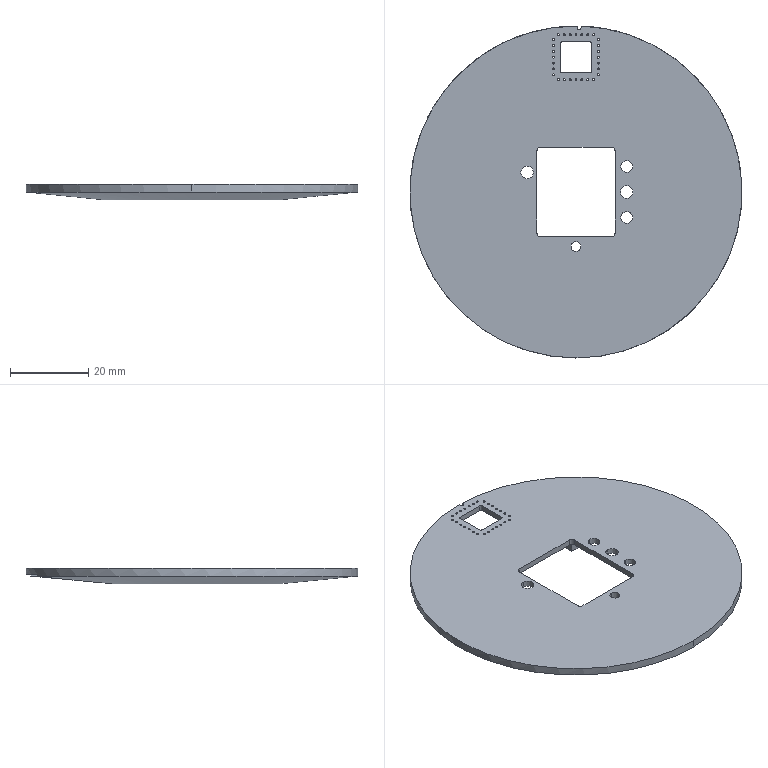Part | 1 solid | 124 faces | box 85 x 85 x 4 mm | volume 14241 mm3 | cylinder 92 | plane 31 | cone 1 | commonest cylinder face diameters 0.5 x56 2 x17 1 x6 3 x4 3.2 x4 85 x3